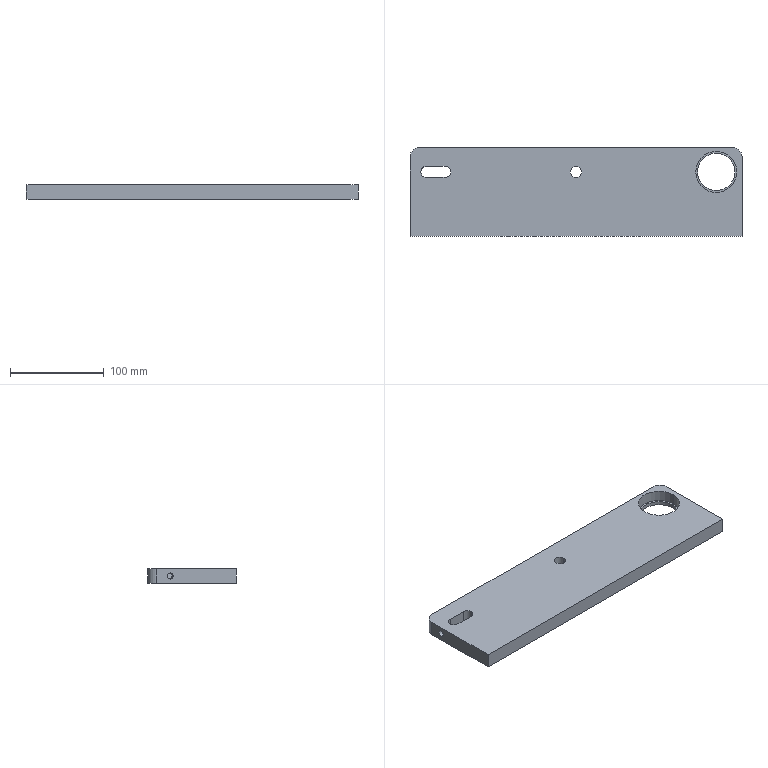Part | STEP file | Flat belt mounting plate | 1 solid | 22 faces | box 355 x 95 x 16 mm | volume 507779 mm3 | cylinder 13 | plane 9 | commonest cylinder face diameters 12 x5 6.5 x2 20 x2 40 x2 44 x2
STEP:
#1=CARTESIAN_POINT('',(128.,21.5,-4.));
#2=VERTEX_POINT('',#1);
#3=CARTESIAN_POINT('',(172.,21.5,-4.));
#4=VERTEX_POINT('',#3);
#5=CARTESIAN_POINT('',(150.,21.5,-4.));
#6=DIRECTION('',(0.,0.,1.));
#7=DIRECTION('',(1.,0.,0.));
#8=AXIS2_PLACEMENT_3D('',#5,#6,#7);
#9=CIRCLE('',#8,22.);
#10=EDGE_CURVE('',#2,#4,#9,.T.);
#11=ORIENTED_EDGE('',*,*,#10,.F.);
#12=CARTESIAN_POINT('',(128.,21.5,8.));
#13=VERTEX_POINT('',#12);
#14=CARTESIAN_POINT('',(128.,21.5,-4.));
#15=DIRECTION('',(0.,0.,1.));
#16=VECTOR('',#15,1000.);
#17=LINE('',#14,#16);
#18=EDGE_CURVE('',#2,#13,#17,.T.);
#19=ORIENTED_EDGE('',*,*,#18,.T.);
#20=CARTESIAN_POINT('',(172.,21.5,8.));
#21=VERTEX_POINT('',#20);
#22=CARTESIAN_POINT('',(150.,21.5,8.));
#23=DIRECTION('',(0.,0.,1.));
#24=DIRECTION('',(1.,0.,0.));
#25=AXIS2_PLACEMENT_3D('',#22,#23,#24);
#26=CIRCLE('',#25,22.);
#27=EDGE_CURVE('',#13,#21,#26,.T.);
#28=ORIENTED_EDGE('',*,*,#27,.T.);
#29=CARTESIAN_POINT('',(172.,21.5,-4.));
#30=DIRECTION('',(0.,0.,1.));
#31=VECTOR('',#30,1000.);
#32=LINE('',#29,#31);
#33=EDGE_CURVE('',#4,#21,#32,.T.);
#34=ORIENTED_EDGE('',*,*,#33,.F.);
#35=EDGE_LOOP('',(#11,#19,#28,#34));
#36=FACE_OUTER_BOUND('',#35,.T.);
#37=CARTESIAN_POINT('',(150.,21.5,-4.));
#38=DIRECTION('',(0.,0.,1.));
#39=DIRECTION('',(1.,0.,0.));
#40=AXIS2_PLACEMENT_3D('',#37,#38,#39);
#41=CYLINDRICAL_SURFACE('',#40,22.);
#42=ADVANCED_FACE('',(#36),#41,.F.);
#43=CARTESIAN_POINT('',(-165.657,23.5,-3.25));
#44=VERTEX_POINT('',#43);
#45=CARTESIAN_POINT('',(-165.657,23.5,3.25));
#46=VERTEX_POINT('',#45);
#47=CARTESIAN_POINT('',(-165.657,23.5,-3.25));
#48=CARTESIAN_POINT('',(-165.729,23.297,-3.25));
#49=CARTESIAN_POINT('',(-165.788,23.093,-3.231));
#50=CARTESIAN_POINT('',(-165.885,22.686,-3.153));
#51=CARTESIAN_POINT('',(-165.923,22.48,-3.093));
#52=CARTESIAN_POINT('',(-165.975,22.085,-2.933));
#53=CARTESIAN_POINT('',(-165.99,21.896,-2.835));
#54=CARTESIAN_POINT('',(-166.003,21.537,-2.599));
#55=CARTESIAN_POINT('',(-166.,21.368,-2.462));
#56=CARTESIAN_POINT('',(-165.986,21.064,-2.162));
#57=CARTESIAN_POINT('',(-165.974,20.926,-1.995));
#58=CARTESIAN_POINT('',(-165.946,20.685,-1.639));
#59=CARTESIAN_POINT('',(-165.93,20.584,-1.452));
#60=CARTESIAN_POINT('',(-165.902,20.419,-1.057));
#61=CARTESIAN_POINT('',(-165.89,20.356,-0.8492));
#62=CARTESIAN_POINT('',(-165.873,20.272,-0.4305));
#63=CARTESIAN_POINT('',(-165.868,20.25,-0.2182));
#64=CARTESIAN_POINT('',(-165.868,20.25,0.2124));
#65=CARTESIAN_POINT('',(-165.873,20.271,0.4277));
#66=CARTESIAN_POINT('',(-165.89,20.355,0.846));
#67=CARTESIAN_POINT('',(-165.902,20.418,1.052));
#68=CARTESIAN_POINT('',(-165.93,20.583,1.449));
#69=CARTESIAN_POINT('',(-165.945,20.684,1.637));
#70=CARTESIAN_POINT('',(-165.973,20.922,1.991));
#71=CARTESIAN_POINT('',(-165.986,21.061,2.159));
#72=CARTESIAN_POINT('',(-166.,21.365,2.46));
#73=CARTESIAN_POINT('',(-166.003,21.53,2.594));
#74=CARTESIAN_POINT('',(-165.99,21.889,2.831));
#75=CARTESIAN_POINT('',(-165.975,22.081,2.932));
#76=CARTESIAN_POINT('',(-165.924,22.473,3.091));
#77=CARTESIAN_POINT('',(-165.887,22.677,3.151));
#78=CARTESIAN_POINT('',(-165.789,23.09,3.231));
#79=CARTESIAN_POINT('',(-165.729,23.296,3.25));
#80=CARTESIAN_POINT('',(-165.657,23.5,3.25));
#81=B_SPLINE_CURVE_WITH_KNOTS('',3,(#47,#48,#49,#50,#51,#52,#53,#54,#55,#56,#57,#58,#59,#60,#61,#62,#63,#64,#65,#66,#67,#68,#69,#70,#71,#72,#73,#74,#75,#76,#77,#78,#79,#80),.UNSPECIFIED.,.F.,.F.,(4,2,2,2,2,2,2,2,2,2,2,2,2,2,2,2,4),(0.01165,0.01228,0.01292,0.01356,0.0142,0.01484,0.01548,0.01612,0.01676,0.0174,0.01804,0.01867,0.01931,0.01995,0.02059,0.02123,0.02187),.UNSPECIFIED.);
#82=EDGE_CURVE('',#44,#46,#81,.T.);
#83=ORIENTED_EDGE('',*,*,#82,.F.);
#84=CARTESIAN_POINT('',(-177.5,23.5,-3.25));
#85=VERTEX_POINT('',#84);
#86=CARTESIAN_POINT('',(-177.5,23.5,-3.25));
#87=DIRECTION('',(-1.,0.,0.));
#88=VECTOR('',#87,1000.);
#89=LINE('',#86,#88);
#90=EDGE_CURVE('',#44,#85,#89,.T.);
#91=ORIENTED_EDGE('',*,*,#90,.T.);
#92=CARTESIAN_POINT('',(-177.5,23.5,3.25));
#93=VERTEX_POINT('',#92);
#94=CARTESIAN_POINT('',(-177.5,23.5,0.));
#95=DIRECTION('',(-1.,0.,0.));
#96=DIRECTION('',(0.,0.,1.));
#97=AXIS2_PLACEMENT_3D('',#94,#95,#96);
#98=CIRCLE('',#97,3.25);
#99=EDGE_CURVE('',#85,#93,#98,.T.);
#100=ORIENTED_EDGE('',*,*,#99,.T.);
#101=CARTESIAN_POINT('',(-177.5,23.5,3.25));
#102=DIRECTION('',(-1.,0.,0.));
#103=VECTOR('',#102,1000.);
#104=LINE('',#101,#103);
#105=EDGE_CURVE('',#46,#93,#104,.T.);
#106=ORIENTED_EDGE('',*,*,#105,.F.);
#107=EDGE_LOOP('',(#83,#91,#100,#106));
#108=FACE_OUTER_BOUND('',#107,.T.);
#109=CARTESIAN_POINT('',(-177.5,23.5,0.));
#110=DIRECTION('',(-1.,0.,0.));
#111=DIRECTION('',(0.,0.,1.));
#112=AXIS2_PLACEMENT_3D('',#109,#110,#111);
#113=CYLINDRICAL_SURFACE('',#112,3.25);
#114=ADVANCED_FACE('',(#108),#113,.F.);
#115=CARTESIAN_POINT('',(-134.,21.5,-8.));
#116=VERTEX_POINT('',#115);
#117=CARTESIAN_POINT('',(-140.,27.5,-8.));
#118=VERTEX_POINT('',#117);
#119=CARTESIAN_POINT('',(-140.,21.5,-8.));
#120=DIRECTION('',(0.,0.,1.));
#121=DIRECTION('',(1.,0.,0.));
#122=AXIS2_PLACEMENT_3D('',#119,#120,#121);
#123=CIRCLE('',#122,6.);
#124=EDGE_CURVE('',#116,#118,#123,.T.);
#125=ORIENTED_EDGE('',*,*,#124,.F.);
#126=CARTESIAN_POINT('',(-134.,21.5,8.));
#127=VERTEX_POINT('',#126);
#128=CARTESIAN_POINT('',(-134.,21.5,-8.));
#129=DIRECTION('',(0.,0.,1.));
#130=VECTOR('',#129,1000.);
#131=LINE('',#128,#130);
#132=EDGE_CURVE('',#116,#127,#131,.T.);
#133=ORIENTED_EDGE('',*,*,#132,.T.);
#134=CARTESIAN_POINT('',(-140.,27.5,8.));
#135=VERTEX_POINT('',#134);
#136=CARTESIAN_POINT('',(-140.,21.5,8.));
#137=DIRECTION('',(0.,0.,1.));
#138=DIRECTION('',(1.,0.,0.));
#139=AXIS2_PLACEMENT_3D('',#136,#137,#138);
#140=CIRCLE('',#139,6.);
#141=EDGE_CURVE('',#127,#135,#140,.T.);
#142=ORIENTED_EDGE('',*,*,#141,.T.);
#143=CARTESIAN_POINT('',(-140.,27.5,-8.));
#144=DIRECTION('',(0.,0.,1.));
#145=VECTOR('',#144,1000.);
#146=LINE('',#143,#145);
#147=EDGE_CURVE('',#118,#135,#146,.T.);
#148=ORIENTED_EDGE('',*,*,#147,.F.);
#149=EDGE_LOOP('',(#125,#133,#142,#148));
#150=FACE_OUTER_BOUND('',#149,.T.);
#151=CARTESIAN_POINT('',(-140.,21.5,-8.));
#152=DIRECTION('',(0.,0.,1.));
#153=DIRECTION('',(1.,0.,0.));
#154=AXIS2_PLACEMENT_3D('',#151,#152,#153);
#155=CYLINDRICAL_SURFACE('',#154,6.);
#156=ADVANCED_FACE('',(#150),#155,.F.);
#157=CARTESIAN_POINT('',(-6.,21.5,-8.));
#158=VERTEX_POINT('',#157);
#159=CARTESIAN_POINT('',(6.,21.5,-8.));
#160=VERTEX_POINT('',#159);
#161=CARTESIAN_POINT('',(0.,21.5,-8.));
#162=DIRECTION('',(0.,0.,1.));
#163=DIRECTION('',(1.,0.,0.));
#164=AXIS2_PLACEMENT_3D('',#161,#162,#163);
#165=CIRCLE('',#164,6.);
#166=EDGE_CURVE('',#158,#160,#165,.T.);
#167=ORIENTED_EDGE('',*,*,#166,.F.);
#168=CARTESIAN_POINT('',(-6.,21.5,8.));
#169=VERTEX_POINT('',#168);
#170=CARTESIAN_POINT('',(-6.,21.5,-8.));
#171=DIRECTION('',(0.,0.,1.));
#172=VECTOR('',#171,1000.);
#173=LINE('',#170,#172);
#174=EDGE_CURVE('',#158,#169,#173,.T.);
#175=ORIENTED_EDGE('',*,*,#174,.T.);
#176=CARTESIAN_POINT('',(6.,21.5,8.));
#177=VERTEX_POINT('',#176);
#178=CARTESIAN_POINT('',(0.,21.5,8.));
#179=DIRECTION('',(0.,0.,1.));
#180=DIRECTION('',(1.,0.,0.));
#181=AXIS2_PLACEMENT_3D('',#178,#179,#180);
#182=CIRCLE('',#181,6.);
#183=EDGE_CURVE('',#169,#177,#182,.T.);
#184=ORIENTED_EDGE('',*,*,#183,.T.);
#185=CARTESIAN_POINT('',(6.,21.5,-8.));
#186=DIRECTION('',(0.,0.,1.));
#187=VECTOR('',#186,1000.);
#188=LINE('',#185,#187);
#189=EDGE_CURVE('',#160,#177,#188,.T.);
#190=ORIENTED_EDGE('',*,*,#189,.F.);
#191=EDGE_LOOP('',(#167,#175,#184,#190));
#192=FACE_OUTER_BOUND('',#191,.T.);
#193=CARTESIAN_POINT('',(0.,21.5,-8.));
#194=DIRECTION('',(0.,0.,1.));
#195=DIRECTION('',(1.,0.,0.));
#196=AXIS2_PLACEMENT_3D('',#193,#194,#195);
#197=CYLINDRICAL_SURFACE('',#196,6.);
#198=ADVANCED_FACE('',(#192),#197,.F.);
#199=CARTESIAN_POINT('',(130.,21.5,-8.));
#200=VERTEX_POINT('',#199);
#201=CARTESIAN_POINT('',(170.,21.5,-8.));
#202=VERTEX_POINT('',#201);
#203=CARTESIAN_POINT('',(150.,21.5,-8.));
#204=DIRECTION('',(0.,0.,1.));
#205=DIRECTION('',(1.,0.,0.));
#206=AXIS2_PLACEMENT_3D('',#203,#204,#205);
#207=CIRCLE('',#206,20.);
#208=EDGE_CURVE('',#200,#202,#207,.T.);
#209=ORIENTED_EDGE('',*,*,#208,.F.);
#210=CARTESIAN_POINT('',(130.,21.5,-4.));
#211=VERTEX_POINT('',#210);
#212=CARTESIAN_POINT('',(130.,21.5,-8.));
#213=DIRECTION('',(0.,0.,1.));
#214=VECTOR('',#213,1000.);
#215=LINE('',#212,#214);
#216=EDGE_CURVE('',#200,#211,#215,.T.);
#217=ORIENTED_EDGE('',*,*,#216,.T.);
#218=CARTESIAN_POINT('',(170.,21.5,-4.));
#219=VERTEX_POINT('',#218);
#220=CARTESIAN_POINT('',(150.,21.5,-4.));
#221=DIRECTION('',(0.,0.,-1.));
#222=DIRECTION('',(1.,0.,0.));
#223=AXIS2_PLACEMENT_3D('',#220,#221,#222);
#224=CIRCLE('',#223,20.);
#225=EDGE_CURVE('',#219,#211,#224,.T.);
#226=ORIENTED_EDGE('',*,*,#225,.F.);
#227=CARTESIAN_POINT('',(170.,21.5,-8.));
#228=DIRECTION('',(0.,0.,1.));
#229=VECTOR('',#228,1000.);
#230=LINE('',#227,#229);
#231=EDGE_CURVE('',#202,#219,#230,.T.);
#232=ORIENTED_EDGE('',*,*,#231,.F.);
#233=EDGE_LOOP('',(#209,#217,#226,#232));
#234=FACE_OUTER_BOUND('',#233,.T.);
#235=CARTESIAN_POINT('',(150.,21.5,-8.));
#236=DIRECTION('',(0.,0.,1.));
#237=DIRECTION('',(1.,0.,0.));
#238=AXIS2_PLACEMENT_3D('',#235,#236,#237);
#239=CYLINDRICAL_SURFACE('',#238,20.);
#240=ADVANCED_FACE('',(#234),#239,.F.);
#241=ORIENTED_EDGE('',*,*,#216,.F.);
#242=CARTESIAN_POINT('',(150.,21.5,-8.));
#243=DIRECTION('',(0.,0.,1.));
#244=DIRECTION('',(1.,0.,0.));
#245=AXIS2_PLACEMENT_3D('',#242,#243,#244);
#246=CIRCLE('',#245,20.);
#247=EDGE_CURVE('',#202,#200,#246,.T.);
#248=ORIENTED_EDGE('',*,*,#247,.F.);
#249=ORIENTED_EDGE('',*,*,#231,.T.);
#250=CARTESIAN_POINT('',(150.,21.5,-4.));
#251=DIRECTION('',(0.,0.,-1.));
#252=DIRECTION('',(1.,0.,0.));
#253=AXIS2_PLACEMENT_3D('',#250,#251,#252);
#254=CIRCLE('',#253,20.);
#255=EDGE_CURVE('',#211,#219,#254,.T.);
#256=ORIENTED_EDGE('',*,*,#255,.F.);
#257=EDGE_LOOP('',(#241,#248,#249,#256));
#258=FACE_OUTER_BOUND('',#257,.T.);
#259=CARTESIAN_POINT('',(150.,21.5,-8.));
#260=DIRECTION('',(0.,0.,1.));
#261=DIRECTION('',(1.,0.,0.));
#262=AXIS2_PLACEMENT_3D('',#259,#260,#261);
#263=CYLINDRICAL_SURFACE('',#262,20.);
#264=ADVANCED_FACE('',(#258),#263,.F.);
#265=CARTESIAN_POINT('',(177.5,-47.5,-8.));
#266=VERTEX_POINT('',#265);
#267=CARTESIAN_POINT('',(177.5,37.5,-8.));
#268=VERTEX_POINT('',#267);
#269=CARTESIAN_POINT('',(177.5,-47.5,-8.));
#270=DIRECTION('',(0.,1.,0.));
#271=VECTOR('',#270,1000.);
#272=LINE('',#269,#271);
#273=EDGE_CURVE('',#266,#268,#272,.T.);
#274=ORIENTED_EDGE('',*,*,#273,.T.);
#275=CARTESIAN_POINT('',(177.5,37.5,8.));
#276=VERTEX_POINT('',#275);
#277=CARTESIAN_POINT('',(177.5,37.5,8.));
#278=DIRECTION('',(0.,0.,1.));
#279=VECTOR('',#278,1000.);
#280=LINE('',#277,#279);
#281=EDGE_CURVE('',#268,#276,#280,.T.);
#282=ORIENTED_EDGE('',*,*,#281,.T.);
#283=CARTESIAN_POINT('',(177.5,-47.5,8.));
#284=VERTEX_POINT('',#283);
#285=CARTESIAN_POINT('',(177.5,-47.5,8.));
#286=DIRECTION('',(0.,1.,0.));
#287=VECTOR('',#286,1000.);
#288=LINE('',#285,#287);
#289=EDGE_CURVE('',#284,#276,#288,.T.);
#290=ORIENTED_EDGE('',*,*,#289,.F.);
#291=CARTESIAN_POINT('',(177.5,-47.5,8.));
#292=DIRECTION('',(0.,0.,-1.));
#293=VECTOR('',#292,1000.);
#294=LINE('',#291,#293);
#295=EDGE_CURVE('',#284,#266,#294,.T.);
#296=ORIENTED_EDGE('',*,*,#295,.T.);
#297=EDGE_LOOP('',(#274,#282,#290,#296));
#298=FACE_OUTER_BOUND('',#297,.T.);
#299=CARTESIAN_POINT('',(177.5,-47.5,8.));
#300=DIRECTION('',(-1.,0.,0.));
#301=DIRECTION('',(0.,0.,1.));
#302=AXIS2_PLACEMENT_3D('',#299,#300,#301);
#303=PLANE('',#302);
#304=ADVANCED_FACE('',(#298),#303,.F.);
#305=CARTESIAN_POINT('',(167.5,47.5,8.));
#306=VERTEX_POINT('',#305);
#307=CARTESIAN_POINT('',(-167.5,47.5,8.));
#308=VERTEX_POINT('',#307);
#309=CARTESIAN_POINT('',(-177.5,47.5,8.));
#310=DIRECTION('',(-1.,0.,0.));
#311=VECTOR('',#310,1000.);
#312=LINE('',#309,#311);
#313=EDGE_CURVE('',#306,#308,#312,.T.);
#314=ORIENTED_EDGE('',*,*,#313,.F.);
#315=CARTESIAN_POINT('',(167.5,47.5,-8.));
#316=VERTEX_POINT('',#315);
#317=CARTESIAN_POINT('',(167.5,47.5,8.));
#318=DIRECTION('',(0.,0.,-1.));
#319=VECTOR('',#318,1000.);
#320=LINE('',#317,#319);
#321=EDGE_CURVE('',#306,#316,#320,.T.);
#322=ORIENTED_EDGE('',*,*,#321,.T.);
#323=CARTESIAN_POINT('',(-167.5,47.5,-8.));
#324=VERTEX_POINT('',#323);
#325=CARTESIAN_POINT('',(-177.5,47.5,-8.));
#326=DIRECTION('',(-1.,0.,0.));
#327=VECTOR('',#326,1000.);
#328=LINE('',#325,#327);
#329=EDGE_CURVE('',#316,#324,#328,.T.);
#330=ORIENTED_EDGE('',*,*,#329,.T.);
#331=CARTESIAN_POINT('',(-167.5,47.5,8.));
#332=DIRECTION('',(0.,0.,1.));
#333=VECTOR('',#332,1000.);
#334=LINE('',#331,#333);
#335=EDGE_CURVE('',#324,#308,#334,.T.);
#336=ORIENTED_EDGE('',*,*,#335,.T.);
#337=EDGE_LOOP('',(#314,#322,#330,#336));
#338=FACE_OUTER_BOUND('',#337,.T.);
#339=CARTESIAN_POINT('',(-177.5,47.5,8.));
#340=DIRECTION('',(0.,-1.,0.));
#341=DIRECTION('',(0.,0.,-1.));
#342=AXIS2_PLACEMENT_3D('',#339,#340,#341);
#343=PLANE('',#342);
#344=ADVANCED_FACE('',(#338),#343,.F.);
#345=CARTESIAN_POINT('',(-177.5,23.5,0.));
#346=DIRECTION('',(-1.,0.,0.));
#347=DIRECTION('',(0.,0.,1.));
#348=AXIS2_PLACEMENT_3D('',#345,#346,#347);
#349=CIRCLE('',#348,3.25);
#350=EDGE_CURVE('',#93,#85,#349,.T.);
#351=ORIENTED_EDGE('',*,*,#350,.F.);
#352=ORIENTED_EDGE('',*,*,#99,.F.);
#353=EDGE_LOOP('',(#351,#352));
#354=FACE_BOUND('',#353,.T.);
#355=CARTESIAN_POINT('',(-177.5,37.5,8.));
#356=VERTEX_POINT('',#355);
#357=CARTESIAN_POINT('',(-177.5,-47.5,8.));
#358=VERTEX_POINT('',#357);
#359=CARTESIAN_POINT('',(-177.5,-47.5,8.));
#360=DIRECTION('',(0.,-1.,0.));
#361=VECTOR('',#360,1000.);
#362=LINE('',#359,#361);
#363=EDGE_CURVE('',#356,#358,#362,.T.);
#364=ORIENTED_EDGE('',*,*,#363,.F.);
#365=CARTESIAN_POINT('',(-177.5,37.5,-8.));
#366=VERTEX_POINT('',#365);
#367=CARTESIAN_POINT('',(-177.5,37.5,8.));
#368=DIRECTION('',(0.,0.,-1.));
#369=VECTOR('',#368,1000.);
#370=LINE('',#367,#369);
#371=EDGE_CURVE('',#356,#366,#370,.T.);
#372=ORIENTED_EDGE('',*,*,#371,.T.);
#373=CARTESIAN_POINT('',(-177.5,-47.5,-8.));
#374=VERTEX_POINT('',#373);
#375=CARTESIAN_POINT('',(-177.5,-47.5,-8.));
#376=DIRECTION('',(0.,-1.,0.));
#377=VECTOR('',#376,1000.);
#378=LINE('',#375,#377);
#379=EDGE_CURVE('',#366,#374,#378,.T.);
#380=ORIENTED_EDGE('',*,*,#379,.T.);
#381=CARTESIAN_POINT('',(-177.5,-47.5,8.));
#382=DIRECTION('',(0.,0.,-1.));
#383=VECTOR('',#382,1000.);
#384=LINE('',#381,#383);
#385=EDGE_CURVE('',#358,#374,#384,.T.);
#386=ORIENTED_EDGE('',*,*,#385,.F.);
#387=EDGE_LOOP('',(#364,#372,#380,#386));
#388=FACE_OUTER_BOUND('',#387,.T.);
#389=CARTESIAN_POINT('',(-177.5,-47.5,8.));
#390=DIRECTION('',(1.,0.,0.));
#391=DIRECTION('',(0.,0.,-1.));
#392=AXIS2_PLACEMENT_3D('',#389,#390,#391);
#393=PLANE('',#392);
#394=ADVANCED_FACE('',(#354,#388),#393,.F.);
#395=CARTESIAN_POINT('',(-177.5,-47.5,-8.));
#396=DIRECTION('',(1.,0.,0.));
#397=VECTOR('',#396,1000.);
#398=LINE('',#395,#397);
#399=EDGE_CURVE('',#374,#266,#398,.T.);
#400=ORIENTED_EDGE('',*,*,#399,.T.);
#401=ORIENTED_EDGE('',*,*,#295,.F.);
#402=CARTESIAN_POINT('',(-177.5,-47.5,8.));
#403=DIRECTION('',(1.,0.,0.));
#404=VECTOR('',#403,1000.);
#405=LINE('',#402,#404);
#406=EDGE_CURVE('',#358,#284,#405,.T.);
#407=ORIENTED_EDGE('',*,*,#406,.F.);
#408=ORIENTED_EDGE('',*,*,#385,.T.);
#409=EDGE_LOOP('',(#400,#401,#407,#408));
#410=FACE_OUTER_BOUND('',#409,.T.);
#411=CARTESIAN_POINT('',(-177.5,-47.5,8.));
#412=DIRECTION('',(0.,1.,0.));
#413=DIRECTION('',(0.,0.,1.));
#414=AXIS2_PLACEMENT_3D('',#411,#412,#413);
#415=PLANE('',#414);
#416=ADVANCED_FACE('',(#410),#415,.F.);
#417=CARTESIAN_POINT('',(150.,21.5,8.));
#418=DIRECTION('',(0.,0.,1.));
#419=DIRECTION('',(1.,0.,0.));
#420=AXIS2_PLACEMENT_3D('',#417,#418,#419);
#421=CIRCLE('',#420,22.);
#422=EDGE_CURVE('',#21,#13,#421,.T.);
#423=ORIENTED_EDGE('',*,*,#422,.F.);
#424=ORIENTED_EDGE('',*,*,#27,.F.);
#425=EDGE_LOOP('',(#423,#424));
#426=FACE_BOUND('',#425,.T.);
#427=CARTESIAN_POINT('',(-160.,15.5,8.));
#428=VERTEX_POINT('',#427);
#429=CARTESIAN_POINT('',(-140.,15.5,8.));
#430=VERTEX_POINT('',#429);
#431=CARTESIAN_POINT('',(-160.,15.5,8.));
#432=DIRECTION('',(1.,0.,0.));
#433=VECTOR('',#432,1000.);
#434=LINE('',#431,#433);
#435=EDGE_CURVE('',#428,#430,#434,.T.);
#436=ORIENTED_EDGE('',*,*,#435,.F.);
#437=CARTESIAN_POINT('',(-160.,27.5,8.));
#438=VERTEX_POINT('',#437);
#439=CARTESIAN_POINT('',(-160.,21.5,8.));
#440=DIRECTION('',(0.,0.,1.));
#441=DIRECTION('',(1.,0.,0.));
#442=AXIS2_PLACEMENT_3D('',#439,#440,#441);
#443=CIRCLE('',#442,6.);
#444=EDGE_CURVE('',#438,#428,#443,.T.);
#445=ORIENTED_EDGE('',*,*,#444,.F.);
#446=CARTESIAN_POINT('',(-160.,27.5,8.));
#447=DIRECTION('',(-1.,0.,0.));
#448=VECTOR('',#447,1000.);
#449=LINE('',#446,#448);
#450=EDGE_CURVE('',#135,#438,#449,.T.);
#451=ORIENTED_EDGE('',*,*,#450,.F.);
#452=ORIENTED_EDGE('',*,*,#141,.F.);
#453=CARTESIAN_POINT('',(-140.,21.5,8.));
#454=DIRECTION('',(0.,0.,1.));
#455=DIRECTION('',(1.,0.,0.));
#456=AXIS2_PLACEMENT_3D('',#453,#454,#455);
#457=CIRCLE('',#456,6.);
#458=EDGE_CURVE('',#430,#127,#457,.T.);
#459=ORIENTED_EDGE('',*,*,#458,.F.);
#460=EDGE_LOOP('',(#436,#445,#451,#452,#459));
#461=FACE_BOUND('',#460,.T.);
#462=CARTESIAN_POINT('',(0.,21.5,8.));
#463=DIRECTION('',(0.,0.,1.));
#464=DIRECTION('',(1.,0.,0.));
#465=AXIS2_PLACEMENT_3D('',#462,#463,#464);
#466=CIRCLE('',#465,6.);
#467=EDGE_CURVE('',#177,#169,#466,.T.);
#468=ORIENTED_EDGE('',*,*,#467,.F.);
#469=ORIENTED_EDGE('',*,*,#183,.F.);
#470=EDGE_LOOP('',(#468,#469));
#471=FACE_BOUND('',#470,.T.);
#472=ORIENTED_EDGE('',*,*,#289,.T.);
#473=CARTESIAN_POINT('',(167.5,37.5,8.));
#474=DIRECTION('',(0.,0.,1.));
#475=DIRECTION('',(-1.,0.,0.));
#476=AXIS2_PLACEMENT_3D('',#473,#474,#475);
#477=CIRCLE('',#476,10.);
#478=EDGE_CURVE('',#276,#306,#477,.T.);
#479=ORIENTED_EDGE('',*,*,#478,.T.);
#480=ORIENTED_EDGE('',*,*,#313,.T.);
#481=CARTESIAN_POINT('',(-167.5,37.5,8.));
#482=DIRECTION('',(0.,0.,1.));
#483=DIRECTION('',(-1.,0.,0.));
#484=AXIS2_PLACEMENT_3D('',#481,#482,#483);
#485=CIRCLE('',#484,10.);
#486=EDGE_CURVE('',#308,#356,#485,.T.);
#487=ORIENTED_EDGE('',*,*,#486,.T.);
#488=ORIENTED_EDGE('',*,*,#363,.T.);
#489=ORIENTED_EDGE('',*,*,#406,.T.);
#490=EDGE_LOOP('',(#472,#479,#480,#487,#488,#489));
#491=FACE_OUTER_BOUND('',#490,.T.);
#492=CARTESIAN_POINT('',(0.,0.,8.));
#493=DIRECTION('',(0.,0.,-1.));
#494=DIRECTION('',(-1.,0.,0.));
#495=AXIS2_PLACEMENT_3D('',#492,#493,#494);
#496=PLANE('',#495);
#497=ADVANCED_FACE('',(#426,#461,#471,#491),#496,.F.);
#498=ORIENTED_EDGE('',*,*,#247,.T.);
#499=ORIENTED_EDGE('',*,*,#208,.T.);
#500=EDGE_LOOP('',(#498,#499));
#501=FACE_BOUND('',#500,.T.);
#502=CARTESIAN_POINT('',(-160.,27.5,-8.));
#503=VERTEX_POINT('',#502);
#504=CARTESIAN_POINT('',(-160.,15.5,-8.));
#505=VERTEX_POINT('',#504);
#506=CARTESIAN_POINT('',(-160.,21.5,-8.));
#507=DIRECTION('',(0.,0.,1.));
#508=DIRECTION('',(1.,0.,0.));
#509=AXIS2_PLACEMENT_3D('',#506,#507,#508);
#510=CIRCLE('',#509,6.);
#511=EDGE_CURVE('',#503,#505,#510,.T.);
#512=ORIENTED_EDGE('',*,*,#511,.T.);
#513=CARTESIAN_POINT('',(-140.,15.5,-8.));
#514=VERTEX_POINT('',#513);
#515=CARTESIAN_POINT('',(-160.,15.5,-8.));
#516=DIRECTION('',(1.,0.,0.));
#517=VECTOR('',#516,1000.);
#518=LINE('',#515,#517);
#519=EDGE_CURVE('',#505,#514,#518,.T.);
#520=ORIENTED_EDGE('',*,*,#519,.T.);
#521=CARTESIAN_POINT('',(-140.,21.5,-8.));
#522=DIRECTION('',(0.,0.,1.));
#523=DIRECTION('',(1.,0.,0.));
#524=AXIS2_PLACEMENT_3D('',#521,#522,#523);
#525=CIRCLE('',#524,6.);
#526=EDGE_CURVE('',#514,#116,#525,.T.);
#527=ORIENTED_EDGE('',*,*,#526,.T.);
#528=ORIENTED_EDGE('',*,*,#124,.T.);
#529=CARTESIAN_POINT('',(-160.,27.5,-8.));
#530=DIRECTION('',(-1.,0.,0.));
#531=VECTOR('',#530,1000.);
#532=LINE('',#529,#531);
#533=EDGE_CURVE('',#118,#503,#532,.T.);
#534=ORIENTED_EDGE('',*,*,#533,.T.);
#535=EDGE_LOOP('',(#512,#520,#527,#528,#534));
#536=FACE_BOUND('',#535,.T.);
#537=CARTESIAN_POINT('',(0.,21.5,-8.));
#538=DIRECTION('',(0.,0.,1.));
#539=DIRECTION('',(1.,0.,0.));
#540=AXIS2_PLACEMENT_3D('',#537,#538,#539);
#541=CIRCLE('',#540,6.);
#542=EDGE_CURVE('',#160,#158,#541,.T.);
#543=ORIENTED_EDGE('',*,*,#542,.T.);
#544=ORIENTED_EDGE('',*,*,#166,.T.);
#545=EDGE_LOOP('',(#543,#544));
#546=FACE_BOUND('',#545,.T.);
#547=ORIENTED_EDGE('',*,*,#329,.F.);
#548=CARTESIAN_POINT('',(167.5,37.5,-8.));
#549=DIRECTION('',(0.,0.,-1.));
#550=DIRECTION('',(-1.,0.,0.));
#551=AXIS2_PLACEMENT_3D('',#548,#549,#550);
#552=CIRCLE('',#551,10.);
#553=EDGE_CURVE('',#316,#268,#552,.T.);
#554=ORIENTED_EDGE('',*,*,#553,.T.);
#555=ORIENTED_EDGE('',*,*,#273,.F.);
#556=ORIENTED_EDGE('',*,*,#399,.F.);
#557=ORIENTED_EDGE('',*,*,#379,.F.);
#558=CARTESIAN_POINT('',(-167.5,37.5,-8.));
#559=DIRECTION('',(0.,0.,-1.));
#560=DIRECTION('',(-1.,0.,0.));
#561=AXIS2_PLACEMENT_3D('',#558,#559,#560);
#562=CIRCLE('',#561,10.);
#563=EDGE_CURVE('',#366,#324,#562,.T.);
#564=ORIENTED_EDGE('',*,*,#563,.T.);
#565=EDGE_LOOP('',(#547,#554,#555,#556,#557,#564));
#566=FACE_OUTER_BOUND('',#565,.T.);
#567=CARTESIAN_POINT('',(0.,0.,-8.));
#568=DIRECTION('',(0.,0.,-1.));
#569=DIRECTION('',(-1.,0.,0.));
#570=AXIS2_PLACEMENT_3D('',#567,#568,#569);
#571=PLANE('',#570);
#572=ADVANCED_FACE('',(#501,#536,#546,#566),#571,.T.);
#573=ORIENTED_EDGE('',*,*,#174,.F.);
#574=ORIENTED_EDGE('',*,*,#542,.F.);
#575=ORIENTED_EDGE('',*,*,#189,.T.);
#576=ORIENTED_EDGE('',*,*,#467,.T.);
#577=EDGE_LOOP('',(#573,#574,#575,#576));
#578=FACE_OUTER_BOUND('',#577,.T.);
#579=CARTESIAN_POINT('',(0.,21.5,-8.));
#580=DIRECTION('',(0.,0.,1.));
#581=DIRECTION('',(1.,0.,0.));
#582=AXIS2_PLACEMENT_3D('',#579,#580,#581);
#583=CYLINDRICAL_SURFACE('',#582,6.);
#584=ADVANCED_FACE('',(#578),#583,.F.);
#585=CARTESIAN_POINT('',(-165.657,23.5,3.25));
#586=CARTESIAN_POINT('',(-165.575,23.733,3.25));
#587=CARTESIAN_POINT('',(-165.48,23.955,3.225));
#588=CARTESIAN_POINT('',(-165.268,24.383,3.135));
#589=CARTESIAN_POINT('',(-165.149,24.589,3.069));
#590=CARTESIAN_POINT('',(-164.897,24.974,2.904));
#591=CARTESIAN_POINT('',(-164.765,25.153,2.805));
#592=CARTESIAN_POINT('',(-164.488,25.488,2.579));
#593=CARTESIAN_POINT('',(-164.345,25.643,2.452));
#594=CARTESIAN_POINT('',(-164.059,25.923,2.175));
#595=CARTESIAN_POINT('',(-163.916,26.05,2.025));
#596=CARTESIAN_POINT('',(-163.633,26.279,1.698));
#597=CARTESIAN_POINT('',(-163.494,26.38,1.521));
#598=CARTESIAN_POINT('',(-163.242,26.551,1.139));
#599=CARTESIAN_POINT('',(-163.126,26.622,0.9309));
#600=CARTESIAN_POINT('',(-162.957,26.722,0.484));
#601=CARTESIAN_POINT('',(-162.904,26.75,0.2398));
#602=CARTESIAN_POINT('',(-162.905,26.75,-0.1274));
#603=CARTESIAN_POINT('',(-162.918,26.742,-0.2514));
#604=CARTESIAN_POINT('',(-162.967,26.715,-0.4896));
#605=CARTESIAN_POINT('',(-163.002,26.695,-0.6061));
#606=CARTESIAN_POINT('',(-163.132,26.619,-0.9434));
#607=CARTESIAN_POINT('',(-163.246,26.548,-1.147));
#608=CARTESIAN_POINT('',(-163.5,26.376,-1.529));
#609=CARTESIAN_POINT('',(-163.639,26.274,-1.704));
#610=CARTESIAN_POINT('',(-163.919,26.047,-2.028));
#611=CARTESIAN_POINT('',(-164.062,25.92,-2.178));
#612=CARTESIAN_POINT('',(-164.349,25.638,-2.455));
#613=CARTESIAN_POINT('',(-164.492,25.484,-2.582));
#614=CARTESIAN_POINT('',(-164.765,25.152,-2.806));
#615=CARTESIAN_POINT('',(-164.897,24.975,-2.904));
#616=CARTESIAN_POINT('',(-165.148,24.591,-3.068));
#617=CARTESIAN_POINT('',(-165.267,24.384,-3.135));
#618=CARTESIAN_POINT('',(-165.48,23.956,-3.225));
#619=CARTESIAN_POINT('',(-165.575,23.732,-3.25));
#620=CARTESIAN_POINT('',(-165.657,23.5,-3.25));
#621=B_SPLINE_CURVE_WITH_KNOTS('',3,(#585,#586,#587,#588,#589,#590,#591,#592,#593,#594,#595,#596,#597,#598,#599,#600,#601,#602,#603,#604,#605,#606,#607,#608,#609,#610,#611,#612,#613,#614,#615,#616,#617,#618,#619,#620),.UNSPECIFIED.,.F.,.F.,(4,2,2,2,2,2,2,2,2,2,2,2,2,2,2,2,2,4),(0.,0.0007279,0.001456,0.002184,0.002911,0.003639,0.004367,0.005095,0.005823,0.006187,0.006551,0.007279,0.008006,0.008734,0.009462,0.01019,0.01092,0.01165),.UNSPECIFIED.);
#622=EDGE_CURVE('',#46,#44,#621,.T.);
#623=ORIENTED_EDGE('',*,*,#622,.T.);
#624=ORIENTED_EDGE('',*,*,#82,.T.);
#625=EDGE_LOOP('',(#623,#624));
#626=FACE_BOUND('',#625,.T.);
#627=ORIENTED_EDGE('',*,*,#444,.T.);
#628=CARTESIAN_POINT('',(-160.,15.5,-8.));
#629=DIRECTION('',(0.,0.,1.));
#630=VECTOR('',#629,1000.);
#631=LINE('',#628,#630);
#632=EDGE_CURVE('',#505,#428,#631,.T.);
#633=ORIENTED_EDGE('',*,*,#632,.F.);
#634=ORIENTED_EDGE('',*,*,#511,.F.);
#635=CARTESIAN_POINT('',(-160.,27.5,-8.));
#636=DIRECTION('',(0.,0.,1.));
#637=VECTOR('',#636,1000.);
#638=LINE('',#635,#637);
#639=EDGE_CURVE('',#503,#438,#638,.T.);
#640=ORIENTED_EDGE('',*,*,#639,.T.);
#641=EDGE_LOOP('',(#627,#633,#634,#640));
#642=FACE_OUTER_BOUND('',#641,.T.);
#643=CARTESIAN_POINT('',(-160.,21.5,-8.));
#644=DIRECTION('',(0.,0.,1.));
#645=DIRECTION('',(1.,0.,0.));
#646=AXIS2_PLACEMENT_3D('',#643,#644,#645);
#647=CYLINDRICAL_SURFACE('',#646,6.);
#648=ADVANCED_FACE('',(#626,#642),#647,.F.);
#649=ORIENTED_EDGE('',*,*,#450,.T.);
#650=ORIENTED_EDGE('',*,*,#639,.F.);
#651=ORIENTED_EDGE('',*,*,#533,.F.);
#652=ORIENTED_EDGE('',*,*,#147,.T.);
#653=EDGE_LOOP('',(#649,#650,#651,#652));
#654=FACE_OUTER_BOUND('',#653,.T.);
#655=CARTESIAN_POINT('',(-160.,27.5,-8.));
#656=DIRECTION('',(0.,1.,0.));
#657=DIRECTION('',(-1.,0.,0.));
#658=AXIS2_PLACEMENT_3D('',#655,#656,#657);
#659=PLANE('',#658);
#660=ADVANCED_FACE('',(#654),#659,.F.);
#661=ORIENTED_EDGE('',*,*,#132,.F.);
#662=ORIENTED_EDGE('',*,*,#526,.F.);
#663=CARTESIAN_POINT('',(-140.,15.5,-8.));
#664=DIRECTION('',(0.,0.,1.));
#665=VECTOR('',#664,1000.);
#666=LINE('',#663,#665);
#667=EDGE_CURVE('',#514,#430,#666,.T.);
#668=ORIENTED_EDGE('',*,*,#667,.T.);
#669=ORIENTED_EDGE('',*,*,#458,.T.);
#670=EDGE_LOOP('',(#661,#662,#668,#669));
#671=FACE_OUTER_BOUND('',#670,.T.);
#672=CARTESIAN_POINT('',(-140.,21.5,-8.));
#673=DIRECTION('',(0.,0.,1.));
#674=DIRECTION('',(1.,0.,0.));
#675=AXIS2_PLACEMENT_3D('',#672,#673,#674);
#676=CYLINDRICAL_SURFACE('',#675,6.);
#677=ADVANCED_FACE('',(#671),#676,.F.);
#678=ORIENTED_EDGE('',*,*,#435,.T.);
#679=ORIENTED_EDGE('',*,*,#667,.F.);
#680=ORIENTED_EDGE('',*,*,#519,.F.);
#681=ORIENTED_EDGE('',*,*,#632,.T.);
#682=EDGE_LOOP('',(#678,#679,#680,#681));
#683=FACE_OUTER_BOUND('',#682,.T.);
#684=CARTESIAN_POINT('',(-160.,15.5,-8.));
#685=DIRECTION('',(0.,-1.,0.));
#686=DIRECTION('',(1.,0.,0.));
#687=AXIS2_PLACEMENT_3D('',#684,#685,#686);
#688=PLANE('',#687);
#689=ADVANCED_FACE('',(#683),#688,.F.);
#690=ORIENTED_EDGE('',*,*,#90,.F.);
#691=ORIENTED_EDGE('',*,*,#622,.F.);
#692=ORIENTED_EDGE('',*,*,#105,.T.);
#693=ORIENTED_EDGE('',*,*,#350,.T.);
#694=EDGE_LOOP('',(#690,#691,#692,#693));
#695=FACE_OUTER_BOUND('',#694,.T.);
#696=CARTESIAN_POINT('',(-177.5,23.5,0.));
#697=DIRECTION('',(-1.,0.,0.));
#698=DIRECTION('',(0.,0.,1.));
#699=AXIS2_PLACEMENT_3D('',#696,#697,#698);
#700=CYLINDRICAL_SURFACE('',#699,3.25);
#701=ADVANCED_FACE('',(#695),#700,.F.);
#702=CARTESIAN_POINT('',(150.,21.5,-4.));
#703=DIRECTION('',(0.,0.,1.));
#704=DIRECTION('',(1.,0.,0.));
#705=AXIS2_PLACEMENT_3D('',#702,#703,#704);
#706=CIRCLE('',#705,22.);
#707=EDGE_CURVE('',#4,#2,#706,.T.);
#708=ORIENTED_EDGE('',*,*,#707,.T.);
#709=ORIENTED_EDGE('',*,*,#10,.T.);
#710=EDGE_LOOP('',(#708,#709));
#711=FACE_OUTER_BOUND('',#710,.T.);
#712=ORIENTED_EDGE('',*,*,#225,.T.);
#713=ORIENTED_EDGE('',*,*,#255,.T.);
#714=EDGE_LOOP('',(#712,#713));
#715=FACE_BOUND('',#714,.T.);
#716=CARTESIAN_POINT('',(150.,21.5,-4.));
#717=DIRECTION('',(0.,0.,1.));
#718=DIRECTION('',(1.,0.,0.));
#719=AXIS2_PLACEMENT_3D('',#716,#717,#718);
#720=PLANE('',#719);
#721=ADVANCED_FACE('',(#711,#715),#720,.T.);
#722=ORIENTED_EDGE('',*,*,#18,.F.);
#723=ORIENTED_EDGE('',*,*,#707,.F.);
#724=ORIENTED_EDGE('',*,*,#33,.T.);
#725=ORIENTED_EDGE('',*,*,#422,.T.);
#726=EDGE_LOOP('',(#722,#723,#724,#725));
#727=FACE_OUTER_BOUND('',#726,.T.);
#728=CARTESIAN_POINT('',(150.,21.5,-4.));
#729=DIRECTION('',(0.,0.,1.));
#730=DIRECTION('',(1.,0.,0.));
#731=AXIS2_PLACEMENT_3D('',#728,#729,#730);
#732=CYLINDRICAL_SURFACE('',#731,22.);
#733=ADVANCED_FACE('',(#727),#732,.F.);
#734=ORIENTED_EDGE('',*,*,#478,.F.);
#735=ORIENTED_EDGE('',*,*,#281,.F.);
#736=ORIENTED_EDGE('',*,*,#553,.F.);
#737=ORIENTED_EDGE('',*,*,#321,.F.);
#738=EDGE_LOOP('',(#734,#735,#736,#737));
#739=FACE_OUTER_BOUND('',#738,.T.);
#740=CARTESIAN_POINT('',(167.5,37.5,8.));
#741=DIRECTION('',(0.,0.,-1.));
#742=DIRECTION('',(-1.,0.,0.));
#743=AXIS2_PLACEMENT_3D('',#740,#741,#742);
#744=CYLINDRICAL_SURFACE('',#743,10.);
#745=ADVANCED_FACE('',(#739),#744,.T.);
#746=ORIENTED_EDGE('',*,*,#486,.F.);
#747=ORIENTED_EDGE('',*,*,#335,.F.);
#748=ORIENTED_EDGE('',*,*,#563,.F.);
#749=ORIENTED_EDGE('',*,*,#371,.F.);
#750=EDGE_LOOP('',(#746,#747,#748,#749));
#751=FACE_OUTER_BOUND('',#750,.T.);
#752=CARTESIAN_POINT('',(-167.5,37.5,8.));
#753=DIRECTION('',(0.,0.,-1.));
#754=DIRECTION('',(-1.,0.,0.));
#755=AXIS2_PLACEMENT_3D('',#752,#753,#754);
#756=CYLINDRICAL_SURFACE('',#755,10.);
#757=ADVANCED_FACE('',(#751),#756,.T.);
#758=CLOSED_SHELL('',(#42,#114,#156,#198,#240,#264,#304,#344,#394,#416,#497,#572,#584,#648,#660,#677,#689,#701,#721,#733,#745,#757));
#759=MANIFOLD_SOLID_BREP('',#758);
#760=CARTESIAN_POINT('',(0.,0.,0.));
#761=DIRECTION('',(0.,0.,1.));
#762=DIRECTION('',(1.,0.,0.));
#763=AXIS2_PLACEMENT_3D('',#760,#761,#762);
#764=(LENGTH_UNIT()NAMED_UNIT(*)SI_UNIT(.MILLI.,.METRE.));
#765=UNCERTAINTY_MEASURE_WITH_UNIT(LENGTH_MEASURE(0.00001),#764,'','');
#766=(NAMED_UNIT(*)PLANE_ANGLE_UNIT()SI_UNIT($,.RADIAN.));
#767=(NAMED_UNIT(*)SI_UNIT($,.STERADIAN.)SOLID_ANGLE_UNIT());
#768=(GEOMETRIC_REPRESENTATION_CONTEXT(3)GLOBAL_UNCERTAINTY_ASSIGNED_CONTEXT((#765))GLOBAL_UNIT_ASSIGNED_CONTEXT((#764,#766,#767))REPRESENTATION_CONTEXT('',''));
#769=ADVANCED_BREP_SHAPE_REPRESENTATION('',(#759,#763),#768);